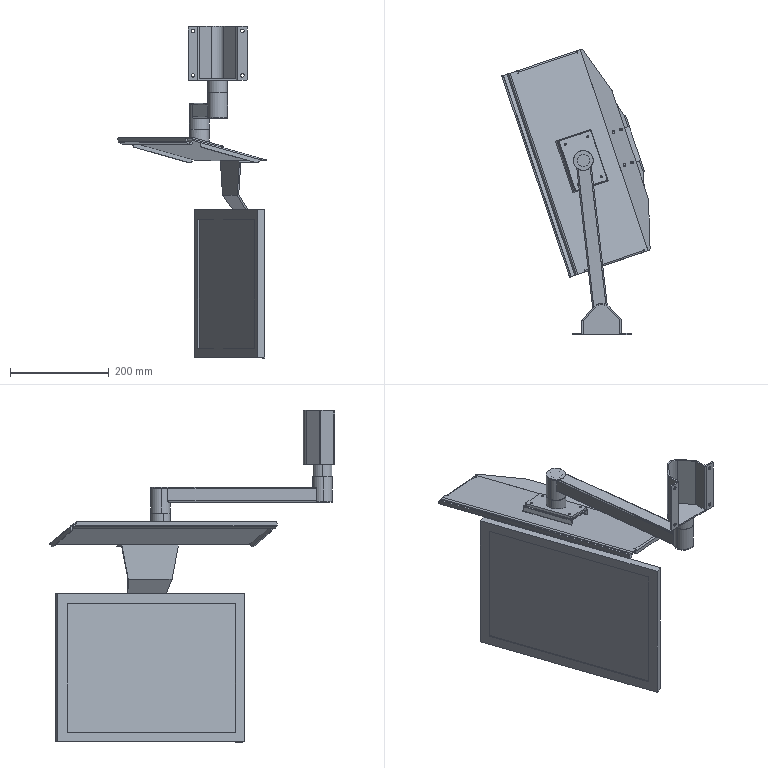Part | SolidWorks | 18 solids | 370 faces | box 300.234 x 578.209 x 672.62 mm | volume 4364638 mm3 | plane 190 | cylinder 166 | cone 12 | spline 2 | commonest cylinder face diameters 0.4 x18 4.2 x16 8 x16 40 x16 6 x12 6.4 x10